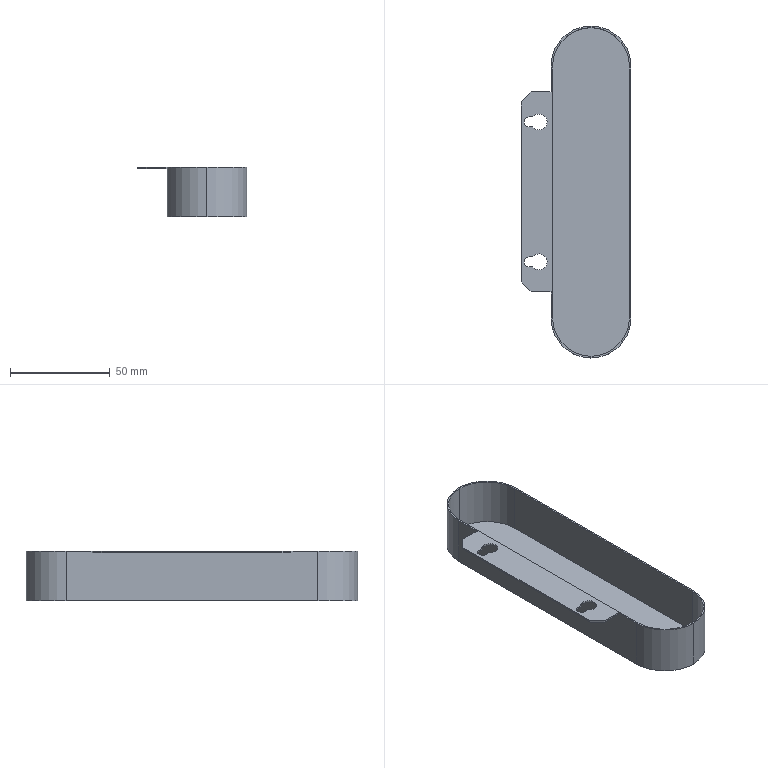Part | NX | features BREP 1 | 1 solid | 31 faces | box 55 x 166 x 25 mm | volume 13374 mm3 | plane 17 | cylinder 14 | commonest cylinder face diameters 5 x4 38.4 x4 40 x4 8 x2
STEP:
#1=CARTESIAN_POINT('',(-31.,-32.5,12.5));
#2=VERTEX_POINT('',#1);
#3=CARTESIAN_POINT('',(-33.5,-35.,12.5));
#4=VERTEX_POINT('',#3);
#5=CARTESIAN_POINT('',(-31.,-35.,12.5));
#6=DIRECTION('',(0.,0.,1.));
#7=DIRECTION('',(-1.,0.,0.));
#8=AXIS2_PLACEMENT_3D('',#5,#6,#7);
#9=CIRCLE('',#8,2.5);
#10=EDGE_CURVE('',#2,#4,#9,.T.);
#11=ORIENTED_EDGE('',*,*,#10,.T.);
#12=CARTESIAN_POINT('',(-33.5,-35.,11.7));
#13=VERTEX_POINT('',#12);
#14=CARTESIAN_POINT('',(-33.5,-35.,12.5));
#15=DIRECTION('',(0.,0.,-1.));
#16=VECTOR('',#15,1000.);
#17=LINE('',#14,#16);
#18=EDGE_CURVE('',#4,#13,#17,.T.);
#19=ORIENTED_EDGE('',*,*,#18,.T.);
#20=CARTESIAN_POINT('',(-31.,-32.5,11.7));
#21=VERTEX_POINT('',#20);
#22=CARTESIAN_POINT('',(-31.,-35.,11.7));
#23=DIRECTION('',(0.,0.,1.));
#24=DIRECTION('',(-1.,0.,0.));
#25=AXIS2_PLACEMENT_3D('',#22,#23,#24);
#26=CIRCLE('',#25,2.5);
#27=EDGE_CURVE('',#21,#13,#26,.T.);
#28=ORIENTED_EDGE('',*,*,#27,.F.);
#29=CARTESIAN_POINT('',(-31.,-32.5,12.5));
#30=DIRECTION('',(0.,0.,-1.));
#31=VECTOR('',#30,1000.);
#32=LINE('',#29,#31);
#33=EDGE_CURVE('',#2,#21,#32,.T.);
#34=ORIENTED_EDGE('',*,*,#33,.F.);
#35=EDGE_LOOP('',(#11,#19,#28,#34));
#36=FACE_BOUND('',#35,.T.);
#37=CARTESIAN_POINT('',(-31.,-35.,12.5));
#38=DIRECTION('',(0.,0.,-1.));
#39=DIRECTION('',(-1.,0.,0.));
#40=AXIS2_PLACEMENT_3D('',#37,#38,#39);
#41=CYLINDRICAL_SURFACE('',#40,2.5);
#42=ADVANCED_FACE('',(#36),#41,.F.);
#43=CARTESIAN_POINT('',(-33.5,35.,12.5));
#44=VERTEX_POINT('',#43);
#45=CARTESIAN_POINT('',(-31.,37.5,12.5));
#46=VERTEX_POINT('',#45);
#47=CARTESIAN_POINT('',(-31.,35.,12.5));
#48=DIRECTION('',(0.,0.,-1.));
#49=DIRECTION('',(-1.,0.,0.));
#50=AXIS2_PLACEMENT_3D('',#47,#48,#49);
#51=CIRCLE('',#50,2.5);
#52=EDGE_CURVE('',#44,#46,#51,.T.);
#53=ORIENTED_EDGE('',*,*,#52,.F.);
#54=CARTESIAN_POINT('',(-33.5,35.,11.7));
#55=VERTEX_POINT('',#54);
#56=CARTESIAN_POINT('',(-33.5,35.,12.5));
#57=DIRECTION('',(0.,0.,-1.));
#58=VECTOR('',#57,1000.);
#59=LINE('',#56,#58);
#60=EDGE_CURVE('',#44,#55,#59,.T.);
#61=ORIENTED_EDGE('',*,*,#60,.T.);
#62=CARTESIAN_POINT('',(-31.,37.5,11.7));
#63=VERTEX_POINT('',#62);
#64=CARTESIAN_POINT('',(-31.,35.,11.7));
#65=DIRECTION('',(0.,0.,-1.));
#66=DIRECTION('',(-1.,0.,0.));
#67=AXIS2_PLACEMENT_3D('',#64,#65,#66);
#68=CIRCLE('',#67,2.5);
#69=EDGE_CURVE('',#55,#63,#68,.T.);
#70=ORIENTED_EDGE('',*,*,#69,.T.);
#71=CARTESIAN_POINT('',(-31.,37.5,12.5));
#72=DIRECTION('',(0.,0.,-1.));
#73=VECTOR('',#72,1000.);
#74=LINE('',#71,#73);
#75=EDGE_CURVE('',#46,#63,#74,.T.);
#76=ORIENTED_EDGE('',*,*,#75,.F.);
#77=EDGE_LOOP('',(#53,#61,#70,#76));
#78=FACE_BOUND('',#77,.T.);
#79=CARTESIAN_POINT('',(-31.,35.,12.5));
#80=DIRECTION('',(0.,0.,-1.));
#81=DIRECTION('',(-1.,0.,0.));
#82=AXIS2_PLACEMENT_3D('',#79,#80,#81);
#83=CYLINDRICAL_SURFACE('',#82,2.5);
#84=ADVANCED_FACE('',(#78),#83,.F.);
#85=CARTESIAN_POINT('',(-35.,-45.,12.5));
#86=VERTEX_POINT('',#85);
#87=CARTESIAN_POINT('',(-35.,45.,12.5));
#88=VERTEX_POINT('',#87);
#89=CARTESIAN_POINT('',(-35.,50.,12.5));
#90=DIRECTION('',(0.,1.,0.));
#91=VECTOR('',#90,1000.);
#92=LINE('',#89,#91);
#93=EDGE_CURVE('',#86,#88,#92,.T.);
#94=ORIENTED_EDGE('',*,*,#93,.F.);
#95=CARTESIAN_POINT('',(-30.,-50.,12.5));
#96=VERTEX_POINT('',#95);
#97=CARTESIAN_POINT('',(-35.,-45.,12.5));
#98=DIRECTION('',(0.7071,-0.7071,0.));
#99=VECTOR('',#98,1000.);
#100=LINE('',#97,#99);
#101=EDGE_CURVE('',#86,#96,#100,.T.);
#102=ORIENTED_EDGE('',*,*,#101,.T.);
#103=CARTESIAN_POINT('',(-20.,-50.,12.5));
#104=VERTEX_POINT('',#103);
#105=CARTESIAN_POINT('',(-35.,-50.,12.5));
#106=DIRECTION('',(1.,0.,0.));
#107=VECTOR('',#106,1000.);
#108=LINE('',#105,#107);
#109=EDGE_CURVE('',#96,#104,#108,.T.);
#110=ORIENTED_EDGE('',*,*,#109,.T.);
#111=CARTESIAN_POINT('',(-20.,-63.,12.5));
#112=VERTEX_POINT('',#111);
#113=CARTESIAN_POINT('',(-20.,83.,12.5));
#114=DIRECTION('',(0.,-1.,0.));
#115=VECTOR('',#114,1000.);
#116=LINE('',#113,#115);
#117=EDGE_CURVE('',#104,#112,#116,.T.);
#118=ORIENTED_EDGE('',*,*,#117,.T.);
#119=CARTESIAN_POINT('',(0.,-83.,12.5));
#120=VERTEX_POINT('',#119);
#121=CARTESIAN_POINT('',(0.,-63.,12.5));
#122=DIRECTION('',(0.,0.,1.));
#123=DIRECTION('',(-1.,0.,0.));
#124=AXIS2_PLACEMENT_3D('',#121,#122,#123);
#125=CIRCLE('',#124,20.);
#126=EDGE_CURVE('',#112,#120,#125,.T.);
#127=ORIENTED_EDGE('',*,*,#126,.T.);
#128=CARTESIAN_POINT('',(20.,-63.,12.5));
#129=VERTEX_POINT('',#128);
#130=CARTESIAN_POINT('',(0.,-63.,12.5));
#131=DIRECTION('',(0.,0.,1.));
#132=DIRECTION('',(-1.,0.,0.));
#133=AXIS2_PLACEMENT_3D('',#130,#131,#132);
#134=CIRCLE('',#133,20.);
#135=EDGE_CURVE('',#120,#129,#134,.T.);
#136=ORIENTED_EDGE('',*,*,#135,.T.);
#137=CARTESIAN_POINT('',(20.,63.,12.5));
#138=VERTEX_POINT('',#137);
#139=CARTESIAN_POINT('',(20.,83.,12.5));
#140=DIRECTION('',(0.,-1.,0.));
#141=VECTOR('',#140,1000.);
#142=LINE('',#139,#141);
#143=EDGE_CURVE('',#138,#129,#142,.T.);
#144=ORIENTED_EDGE('',*,*,#143,.F.);
#145=CARTESIAN_POINT('',(0.,83.,12.5));
#146=VERTEX_POINT('',#145);
#147=CARTESIAN_POINT('',(0.,63.,12.5));
#148=DIRECTION('',(0.,0.,1.));
#149=DIRECTION('',(-1.,0.,0.));
#150=AXIS2_PLACEMENT_3D('',#147,#148,#149);
#151=CIRCLE('',#150,20.);
#152=EDGE_CURVE('',#138,#146,#151,.T.);
#153=ORIENTED_EDGE('',*,*,#152,.T.);
#154=CARTESIAN_POINT('',(-20.,63.,12.5));
#155=VERTEX_POINT('',#154);
#156=CARTESIAN_POINT('',(0.,63.,12.5));
#157=DIRECTION('',(0.,0.,1.));
#158=DIRECTION('',(-1.,0.,0.));
#159=AXIS2_PLACEMENT_3D('',#156,#157,#158);
#160=CIRCLE('',#159,20.);
#161=EDGE_CURVE('',#146,#155,#160,.T.);
#162=ORIENTED_EDGE('',*,*,#161,.T.);
#163=CARTESIAN_POINT('',(-20.,50.,12.5));
#164=VERTEX_POINT('',#163);
#165=CARTESIAN_POINT('',(-20.,83.,12.5));
#166=DIRECTION('',(0.,-1.,0.));
#167=VECTOR('',#166,1000.);
#168=LINE('',#165,#167);
#169=EDGE_CURVE('',#155,#164,#168,.T.);
#170=ORIENTED_EDGE('',*,*,#169,.T.);
#171=CARTESIAN_POINT('',(-30.,50.,12.5));
#172=VERTEX_POINT('',#171);
#173=CARTESIAN_POINT('',(-35.,50.,12.5));
#174=DIRECTION('',(1.,0.,0.));
#175=VECTOR('',#174,1000.);
#176=LINE('',#173,#175);
#177=EDGE_CURVE('',#172,#164,#176,.T.);
#178=ORIENTED_EDGE('',*,*,#177,.F.);
#179=CARTESIAN_POINT('',(-35.,45.,12.5));
#180=DIRECTION('',(-0.7071,-0.7071,0.));
#181=VECTOR('',#180,1000.);
#182=LINE('',#179,#181);
#183=EDGE_CURVE('',#172,#88,#182,.T.);
#184=ORIENTED_EDGE('',*,*,#183,.T.);
#185=EDGE_LOOP('',(#94,#102,#110,#118,#127,#136,#144,#153,#162,#170,#178,#184));
#186=FACE_BOUND('',#185,.T.);
#187=CARTESIAN_POINT('',(-29.122,37.5,12.5));
#188=VERTEX_POINT('',#187);
#189=CARTESIAN_POINT('',(0.,37.5,12.5));
#190=DIRECTION('',(-1.,0.,0.));
#191=VECTOR('',#190,1000.);
#192=LINE('',#189,#191);
#193=EDGE_CURVE('',#188,#46,#192,.T.);
#194=ORIENTED_EDGE('',*,*,#193,.F.);
#195=CARTESIAN_POINT('',(-29.122,32.5,12.5));
#196=VERTEX_POINT('',#195);
#197=CARTESIAN_POINT('',(-26.,35.,12.5));
#198=DIRECTION('',(0.,0.,-1.));
#199=DIRECTION('',(-1.,0.,0.));
#200=AXIS2_PLACEMENT_3D('',#197,#198,#199);
#201=CIRCLE('',#200,4.);
#202=EDGE_CURVE('',#188,#196,#201,.T.);
#203=ORIENTED_EDGE('',*,*,#202,.T.);
#204=CARTESIAN_POINT('',(-31.,32.5,12.5));
#205=VERTEX_POINT('',#204);
#206=CARTESIAN_POINT('',(0.,32.5,12.5));
#207=DIRECTION('',(-1.,0.,0.));
#208=VECTOR('',#207,1000.);
#209=LINE('',#206,#208);
#210=EDGE_CURVE('',#196,#205,#209,.T.);
#211=ORIENTED_EDGE('',*,*,#210,.T.);
#212=CARTESIAN_POINT('',(-31.,35.,12.5));
#213=DIRECTION('',(0.,0.,-1.));
#214=DIRECTION('',(-1.,0.,0.));
#215=AXIS2_PLACEMENT_3D('',#212,#213,#214);
#216=CIRCLE('',#215,2.5);
#217=EDGE_CURVE('',#205,#44,#216,.T.);
#218=ORIENTED_EDGE('',*,*,#217,.T.);
#219=ORIENTED_EDGE('',*,*,#52,.T.);
#220=EDGE_LOOP('',(#194,#203,#211,#218,#219));
#221=FACE_BOUND('',#220,.T.);
#222=CARTESIAN_POINT('',(-19.2,-63.,12.5));
#223=VERTEX_POINT('',#222);
#224=CARTESIAN_POINT('',(0.,-82.2,12.5));
#225=VERTEX_POINT('',#224);
#226=CARTESIAN_POINT('',(0.,-63.,12.5));
#227=DIRECTION('',(0.,0.,1.));
#228=DIRECTION('',(-1.,0.,0.));
#229=AXIS2_PLACEMENT_3D('',#226,#227,#228);
#230=CIRCLE('',#229,19.2);
#231=EDGE_CURVE('',#223,#225,#230,.T.);
#232=ORIENTED_EDGE('',*,*,#231,.F.);
#233=CARTESIAN_POINT('',(-19.2,63.,12.5));
#234=VERTEX_POINT('',#233);
#235=CARTESIAN_POINT('',(-19.2,83.,12.5));
#236=DIRECTION('',(0.,-1.,0.));
#237=VECTOR('',#236,1000.);
#238=LINE('',#235,#237);
#239=EDGE_CURVE('',#234,#223,#238,.T.);
#240=ORIENTED_EDGE('',*,*,#239,.F.);
#241=CARTESIAN_POINT('',(0.,82.2,12.5));
#242=VERTEX_POINT('',#241);
#243=CARTESIAN_POINT('',(0.,63.,12.5));
#244=DIRECTION('',(0.,0.,1.));
#245=DIRECTION('',(-1.,0.,0.));
#246=AXIS2_PLACEMENT_3D('',#243,#244,#245);
#247=CIRCLE('',#246,19.2);
#248=EDGE_CURVE('',#242,#234,#247,.T.);
#249=ORIENTED_EDGE('',*,*,#248,.F.);
#250=CARTESIAN_POINT('',(19.2,63.,12.5));
#251=VERTEX_POINT('',#250);
#252=CARTESIAN_POINT('',(0.,63.,12.5));
#253=DIRECTION('',(0.,0.,1.));
#254=DIRECTION('',(-1.,0.,0.));
#255=AXIS2_PLACEMENT_3D('',#252,#253,#254);
#256=CIRCLE('',#255,19.2);
#257=EDGE_CURVE('',#251,#242,#256,.T.);
#258=ORIENTED_EDGE('',*,*,#257,.F.);
#259=CARTESIAN_POINT('',(19.2,-63.,12.5));
#260=VERTEX_POINT('',#259);
#261=CARTESIAN_POINT('',(19.2,83.,12.5));
#262=DIRECTION('',(0.,-1.,0.));
#263=VECTOR('',#262,1000.);
#264=LINE('',#261,#263);
#265=EDGE_CURVE('',#251,#260,#264,.T.);
#266=ORIENTED_EDGE('',*,*,#265,.T.);
#267=CARTESIAN_POINT('',(0.,-63.,12.5));
#268=DIRECTION('',(0.,0.,1.));
#269=DIRECTION('',(-1.,0.,0.));
#270=AXIS2_PLACEMENT_3D('',#267,#268,#269);
#271=CIRCLE('',#270,19.2);
#272=EDGE_CURVE('',#225,#260,#271,.T.);
#273=ORIENTED_EDGE('',*,*,#272,.F.);
#274=EDGE_LOOP('',(#232,#240,#249,#258,#266,#273));
#275=FACE_BOUND('',#274,.T.);
#276=CARTESIAN_POINT('',(-29.122,-32.5,12.5));
#277=VERTEX_POINT('',#276);
#278=CARTESIAN_POINT('',(0.,-32.5,12.5));
#279=DIRECTION('',(-1.,0.,0.));
#280=VECTOR('',#279,1000.);
#281=LINE('',#278,#280);
#282=EDGE_CURVE('',#277,#2,#281,.T.);
#283=ORIENTED_EDGE('',*,*,#282,.F.);
#284=CARTESIAN_POINT('',(-29.122,-37.5,12.5));
#285=VERTEX_POINT('',#284);
#286=CARTESIAN_POINT('',(-26.,-35.,12.5));
#287=DIRECTION('',(0.,0.,1.));
#288=DIRECTION('',(-1.,0.,0.));
#289=AXIS2_PLACEMENT_3D('',#286,#287,#288);
#290=CIRCLE('',#289,4.);
#291=EDGE_CURVE('',#285,#277,#290,.T.);
#292=ORIENTED_EDGE('',*,*,#291,.F.);
#293=CARTESIAN_POINT('',(-31.,-37.5,12.5));
#294=VERTEX_POINT('',#293);
#295=CARTESIAN_POINT('',(0.,-37.5,12.5));
#296=DIRECTION('',(-1.,0.,0.));
#297=VECTOR('',#296,1000.);
#298=LINE('',#295,#297);
#299=EDGE_CURVE('',#285,#294,#298,.T.);
#300=ORIENTED_EDGE('',*,*,#299,.T.);
#301=CARTESIAN_POINT('',(-31.,-35.,12.5));
#302=DIRECTION('',(0.,0.,1.));
#303=DIRECTION('',(-1.,0.,0.));
#304=AXIS2_PLACEMENT_3D('',#301,#302,#303);
#305=CIRCLE('',#304,2.5);
#306=EDGE_CURVE('',#4,#294,#305,.T.);
#307=ORIENTED_EDGE('',*,*,#306,.F.);
#308=ORIENTED_EDGE('',*,*,#10,.F.);
#309=EDGE_LOOP('',(#283,#292,#300,#307,#308));
#310=FACE_BOUND('',#309,.T.);
#311=CARTESIAN_POINT('',(-20.,83.,12.5));
#312=DIRECTION('',(0.,0.,-1.));
#313=DIRECTION('',(0.,-1.,0.));
#314=AXIS2_PLACEMENT_3D('',#311,#312,#313);
#315=PLANE('',#314);
#316=ADVANCED_FACE('',(#186,#221,#275,#310),#315,.F.);
#317=CARTESIAN_POINT('',(-30.,-50.,11.7));
#318=VERTEX_POINT('',#317);
#319=CARTESIAN_POINT('',(-20.,-50.,11.7));
#320=VERTEX_POINT('',#319);
#321=CARTESIAN_POINT('',(-35.,-50.,11.7));
#322=DIRECTION('',(1.,0.,0.));
#323=VECTOR('',#322,1000.);
#324=LINE('',#321,#323);
#325=EDGE_CURVE('',#318,#320,#324,.T.);
#326=ORIENTED_EDGE('',*,*,#325,.F.);
#327=CARTESIAN_POINT('',(-35.,-45.,11.7));
#328=VERTEX_POINT('',#327);
#329=CARTESIAN_POINT('',(-35.,-45.,11.7));
#330=DIRECTION('',(-0.7071,0.7071,0.));
#331=VECTOR('',#330,1000.);
#332=LINE('',#329,#331);
#333=EDGE_CURVE('',#318,#328,#332,.T.);
#334=ORIENTED_EDGE('',*,*,#333,.T.);
#335=CARTESIAN_POINT('',(-35.,45.,11.7));
#336=VERTEX_POINT('',#335);
#337=CARTESIAN_POINT('',(-35.,50.,11.7));
#338=DIRECTION('',(0.,-1.,0.));
#339=VECTOR('',#338,1000.);
#340=LINE('',#337,#339);
#341=EDGE_CURVE('',#336,#328,#340,.T.);
#342=ORIENTED_EDGE('',*,*,#341,.F.);
#343=CARTESIAN_POINT('',(-30.,50.,11.7));
#344=VERTEX_POINT('',#343);
#345=CARTESIAN_POINT('',(-35.,45.,11.7));
#346=DIRECTION('',(0.7071,0.7071,0.));
#347=VECTOR('',#346,1000.);
#348=LINE('',#345,#347);
#349=EDGE_CURVE('',#336,#344,#348,.T.);
#350=ORIENTED_EDGE('',*,*,#349,.T.);
#351=CARTESIAN_POINT('',(-20.,50.,11.7));
#352=VERTEX_POINT('',#351);
#353=CARTESIAN_POINT('',(-35.,50.,11.7));
#354=DIRECTION('',(1.,0.,0.));
#355=VECTOR('',#354,1000.);
#356=LINE('',#353,#355);
#357=EDGE_CURVE('',#344,#352,#356,.T.);
#358=ORIENTED_EDGE('',*,*,#357,.T.);
#359=CARTESIAN_POINT('',(-20.,50.,11.7));
#360=DIRECTION('',(0.,-1.,0.));
#361=VECTOR('',#360,1000.);
#362=LINE('',#359,#361);
#363=EDGE_CURVE('',#352,#320,#362,.T.);
#364=ORIENTED_EDGE('',*,*,#363,.T.);
#365=EDGE_LOOP('',(#326,#334,#342,#350,#358,#364));
#366=FACE_BOUND('',#365,.T.);
#367=CARTESIAN_POINT('',(-29.122,37.5,11.7));
#368=VERTEX_POINT('',#367);
#369=CARTESIAN_POINT('',(0.,37.5,11.7));
#370=DIRECTION('',(-1.,0.,0.));
#371=VECTOR('',#370,1000.);
#372=LINE('',#369,#371);
#373=EDGE_CURVE('',#368,#63,#372,.T.);
#374=ORIENTED_EDGE('',*,*,#373,.T.);
#375=ORIENTED_EDGE('',*,*,#69,.F.);
#376=CARTESIAN_POINT('',(-31.,32.5,11.7));
#377=VERTEX_POINT('',#376);
#378=CARTESIAN_POINT('',(-31.,35.,11.7));
#379=DIRECTION('',(0.,0.,-1.));
#380=DIRECTION('',(-1.,0.,0.));
#381=AXIS2_PLACEMENT_3D('',#378,#379,#380);
#382=CIRCLE('',#381,2.5);
#383=EDGE_CURVE('',#377,#55,#382,.T.);
#384=ORIENTED_EDGE('',*,*,#383,.F.);
#385=CARTESIAN_POINT('',(-29.122,32.5,11.7));
#386=VERTEX_POINT('',#385);
#387=CARTESIAN_POINT('',(0.,32.5,11.7));
#388=DIRECTION('',(-1.,0.,0.));
#389=VECTOR('',#388,1000.);
#390=LINE('',#387,#389);
#391=EDGE_CURVE('',#386,#377,#390,.T.);
#392=ORIENTED_EDGE('',*,*,#391,.F.);
#393=CARTESIAN_POINT('',(-26.,35.,11.7));
#394=DIRECTION('',(0.,0.,-1.));
#395=DIRECTION('',(-1.,0.,0.));
#396=AXIS2_PLACEMENT_3D('',#393,#394,#395);
#397=CIRCLE('',#396,4.);
#398=EDGE_CURVE('',#368,#386,#397,.T.);
#399=ORIENTED_EDGE('',*,*,#398,.F.);
#400=EDGE_LOOP('',(#374,#375,#384,#392,#399));
#401=FACE_BOUND('',#400,.T.);
#402=CARTESIAN_POINT('',(-29.122,-32.5,11.7));
#403=VERTEX_POINT('',#402);
#404=CARTESIAN_POINT('',(0.,-32.5,11.7));
#405=DIRECTION('',(-1.,0.,0.));
#406=VECTOR('',#405,1000.);
#407=LINE('',#404,#406);
#408=EDGE_CURVE('',#403,#21,#407,.T.);
#409=ORIENTED_EDGE('',*,*,#408,.T.);
#410=ORIENTED_EDGE('',*,*,#27,.T.);
#411=CARTESIAN_POINT('',(-31.,-37.5,11.7));
#412=VERTEX_POINT('',#411);
#413=CARTESIAN_POINT('',(-31.,-35.,11.7));
#414=DIRECTION('',(0.,0.,1.));
#415=DIRECTION('',(-1.,0.,0.));
#416=AXIS2_PLACEMENT_3D('',#413,#414,#415);
#417=CIRCLE('',#416,2.5);
#418=EDGE_CURVE('',#13,#412,#417,.T.);
#419=ORIENTED_EDGE('',*,*,#418,.T.);
#420=CARTESIAN_POINT('',(-29.122,-37.5,11.7));
#421=VERTEX_POINT('',#420);
#422=CARTESIAN_POINT('',(0.,-37.5,11.7));
#423=DIRECTION('',(-1.,0.,0.));
#424=VECTOR('',#423,1000.);
#425=LINE('',#422,#424);
#426=EDGE_CURVE('',#421,#412,#425,.T.);
#427=ORIENTED_EDGE('',*,*,#426,.F.);
#428=CARTESIAN_POINT('',(-26.,-35.,11.7));
#429=DIRECTION('',(0.,0.,1.));
#430=DIRECTION('',(-1.,0.,0.));
#431=AXIS2_PLACEMENT_3D('',#428,#429,#430);
#432=CIRCLE('',#431,4.);
#433=EDGE_CURVE('',#421,#403,#432,.T.);
#434=ORIENTED_EDGE('',*,*,#433,.T.);
#435=EDGE_LOOP('',(#409,#410,#419,#427,#434));
#436=FACE_BOUND('',#435,.T.);
#437=CARTESIAN_POINT('',(-35.,50.,11.7));
#438=DIRECTION('',(0.,0.,1.));
#439=DIRECTION('',(1.,0.,0.));
#440=AXIS2_PLACEMENT_3D('',#437,#438,#439);
#441=PLANE('',#440);
#442=ADVANCED_FACE('',(#366,#401,#436),#441,.F.);
#443=CARTESIAN_POINT('',(-20.,50.,12.5));
#444=DIRECTION('',(0.,0.,-1.));
#445=VECTOR('',#444,1000.);
#446=LINE('',#443,#445);
#447=EDGE_CURVE('',#164,#352,#446,.T.);
#448=ORIENTED_EDGE('',*,*,#447,.F.);
#449=ORIENTED_EDGE('',*,*,#169,.F.);
#450=CARTESIAN_POINT('',(-20.,63.,-12.5));
#451=VERTEX_POINT('',#450);
#452=CARTESIAN_POINT('',(-20.,63.,-12.5));
#453=DIRECTION('',(0.,0.,-1.));
#454=VECTOR('',#453,1000.);
#455=LINE('',#452,#454);
#456=EDGE_CURVE('',#155,#451,#455,.T.);
#457=ORIENTED_EDGE('',*,*,#456,.T.);
#458=CARTESIAN_POINT('',(-20.,-63.,-12.5));
#459=VERTEX_POINT('',#458);
#460=CARTESIAN_POINT('',(-20.,83.,-12.5));
#461=DIRECTION('',(0.,-1.,0.));
#462=VECTOR('',#461,1000.);
#463=LINE('',#460,#462);
#464=EDGE_CURVE('',#451,#459,#463,.T.);
#465=ORIENTED_EDGE('',*,*,#464,.T.);
#466=CARTESIAN_POINT('',(-20.,-63.,-12.5));
#467=DIRECTION('',(0.,0.,1.));
#468=VECTOR('',#467,1000.);
#469=LINE('',#466,#468);
#470=EDGE_CURVE('',#459,#112,#469,.T.);
#471=ORIENTED_EDGE('',*,*,#470,.T.);
#472=ORIENTED_EDGE('',*,*,#117,.F.);
#473=CARTESIAN_POINT('',(-20.,-50.,12.5));
#474=DIRECTION('',(0.,0.,1.));
#475=VECTOR('',#474,1000.);
#476=LINE('',#473,#475);
#477=EDGE_CURVE('',#320,#104,#476,.T.);
#478=ORIENTED_EDGE('',*,*,#477,.F.);
#479=ORIENTED_EDGE('',*,*,#363,.F.);
#480=EDGE_LOOP('',(#448,#449,#457,#465,#471,#472,#478,#479));
#481=FACE_BOUND('',#480,.T.);
#482=CARTESIAN_POINT('',(-20.,83.,-12.5));
#483=DIRECTION('',(1.,0.,0.));
#484=DIRECTION('',(0.,1.,0.));
#485=AXIS2_PLACEMENT_3D('',#482,#483,#484);
#486=PLANE('',#485);
#487=ADVANCED_FACE('',(#481),#486,.F.);
#488=ORIENTED_EDGE('',*,*,#143,.T.);
#489=CARTESIAN_POINT('',(20.,-63.,-12.5));
#490=VERTEX_POINT('',#489);
#491=CARTESIAN_POINT('',(20.,-63.,-12.5));
#492=DIRECTION('',(0.,0.,-1.));
#493=VECTOR('',#492,1000.);
#494=LINE('',#491,#493);
#495=EDGE_CURVE('',#129,#490,#494,.T.);
#496=ORIENTED_EDGE('',*,*,#495,.T.);
#497=CARTESIAN_POINT('',(20.,63.,-12.5));
#498=VERTEX_POINT('',#497);
#499=CARTESIAN_POINT('',(20.,83.,-12.5));
#500=DIRECTION('',(0.,-1.,0.));
#501=VECTOR('',#500,1000.);
#502=LINE('',#499,#501);
#503=EDGE_CURVE('',#498,#490,#502,.T.);
#504=ORIENTED_EDGE('',*,*,#503,.F.);
#505=CARTESIAN_POINT('',(20.,63.,12.5));
#506=DIRECTION('',(0.,0.,1.));
#507=VECTOR('',#506,1000.);
#508=LINE('',#505,#507);
#509=EDGE_CURVE('',#498,#138,#508,.T.);
#510=ORIENTED_EDGE('',*,*,#509,.T.);
#511=EDGE_LOOP('',(#488,#496,#504,#510));
#512=FACE_BOUND('',#511,.T.);
#513=CARTESIAN_POINT('',(20.,83.,-12.5));
#514=DIRECTION('',(-1.,0.,0.));
#515=DIRECTION('',(0.,0.,1.));
#516=AXIS2_PLACEMENT_3D('',#513,#514,#515);
#517=PLANE('',#516);
#518=ADVANCED_FACE('',(#512),#517,.F.);
#519=ORIENTED_EDGE('',*,*,#503,.T.);
#520=CARTESIAN_POINT('',(0.,-83.,-12.5));
#521=VERTEX_POINT('',#520);
#522=CARTESIAN_POINT('',(0.,-63.,-12.5));
#523=DIRECTION('',(0.,0.,-1.));
#524=DIRECTION('',(1.,0.,0.));
#525=AXIS2_PLACEMENT_3D('',#522,#523,#524);
#526=CIRCLE('',#525,20.);
#527=EDGE_CURVE('',#490,#521,#526,.T.);
#528=ORIENTED_EDGE('',*,*,#527,.T.);
#529=CARTESIAN_POINT('',(0.,-63.,-12.5));
#530=DIRECTION('',(0.,0.,-1.));
#531=DIRECTION('',(1.,0.,0.));
#532=AXIS2_PLACEMENT_3D('',#529,#530,#531);
#533=CIRCLE('',#532,20.);
#534=EDGE_CURVE('',#521,#459,#533,.T.);
#535=ORIENTED_EDGE('',*,*,#534,.T.);
#536=ORIENTED_EDGE('',*,*,#464,.F.);
#537=CARTESIAN_POINT('',(0.,83.,-12.5));
#538=VERTEX_POINT('',#537);
#539=CARTESIAN_POINT('',(0.,63.,-12.5));
#540=DIRECTION('',(0.,0.,-1.));
#541=DIRECTION('',(1.,0.,0.));
#542=AXIS2_PLACEMENT_3D('',#539,#540,#541);
#543=CIRCLE('',#542,20.);
#544=EDGE_CURVE('',#451,#538,#543,.T.);
#545=ORIENTED_EDGE('',*,*,#544,.T.);
#546=CARTESIAN_POINT('',(0.,63.,-12.5));
#547=DIRECTION('',(0.,0.,-1.));
#548=DIRECTION('',(1.,0.,0.));
#549=AXIS2_PLACEMENT_3D('',#546,#547,#548);
#550=CIRCLE('',#549,20.);
#551=EDGE_CURVE('',#538,#498,#550,.T.);
#552=ORIENTED_EDGE('',*,*,#551,.T.);
#553=EDGE_LOOP('',(#519,#528,#535,#536,#545,#552));
#554=FACE_BOUND('',#553,.T.);
#555=CARTESIAN_POINT('',(-20.,83.,-12.5));
#556=DIRECTION('',(0.,0.,1.));
#557=DIRECTION('',(1.,0.,0.));
#558=AXIS2_PLACEMENT_3D('',#555,#556,#557);
#559=PLANE('',#558);
#560=ADVANCED_FACE('',(#554),#559,.F.);
#561=CARTESIAN_POINT('',(0.,-83.,12.5));
#562=DIRECTION('',(0.,0.,-1.));
#563=VECTOR('',#562,1000.);
#564=LINE('',#561,#563);
#565=EDGE_CURVE('',#120,#521,#564,.T.);
#566=ORIENTED_EDGE('',*,*,#565,.F.);
#567=ORIENTED_EDGE('',*,*,#126,.F.);
#568=ORIENTED_EDGE('',*,*,#470,.F.);
#569=ORIENTED_EDGE('',*,*,#534,.F.);
#570=EDGE_LOOP('',(#566,#567,#568,#569));
#571=FACE_BOUND('',#570,.T.);
#572=CARTESIAN_POINT('',(0.,-63.,-12.5));
#573=DIRECTION('',(0.,0.,1.));
#574=DIRECTION('',(1.,0.,0.));
#575=AXIS2_PLACEMENT_3D('',#572,#573,#574);
#576=CYLINDRICAL_SURFACE('',#575,20.);
#577=ADVANCED_FACE('',(#571),#576,.T.);
#578=ORIENTED_EDGE('',*,*,#135,.F.);
#579=ORIENTED_EDGE('',*,*,#565,.T.);
#580=ORIENTED_EDGE('',*,*,#527,.F.);
#581=ORIENTED_EDGE('',*,*,#495,.F.);
#582=EDGE_LOOP('',(#578,#579,#580,#581));
#583=FACE_BOUND('',#582,.T.);
#584=CARTESIAN_POINT('',(0.,-63.,-12.5));
#585=DIRECTION('',(0.,0.,-1.));
#586=DIRECTION('',(-1.,0.,0.));
#587=AXIS2_PLACEMENT_3D('',#584,#585,#586);
#588=CYLINDRICAL_SURFACE('',#587,20.);
#589=ADVANCED_FACE('',(#583),#588,.T.);
#590=ORIENTED_EDGE('',*,*,#456,.F.);
#591=ORIENTED_EDGE('',*,*,#161,.F.);
#592=CARTESIAN_POINT('',(0.,83.,12.5));
#593=DIRECTION('',(0.,0.,1.));
#594=VECTOR('',#593,1000.);
#595=LINE('',#592,#594);
#596=EDGE_CURVE('',#538,#146,#595,.T.);
#597=ORIENTED_EDGE('',*,*,#596,.F.);
#598=ORIENTED_EDGE('',*,*,#544,.F.);
#599=EDGE_LOOP('',(#590,#591,#597,#598));
#600=FACE_BOUND('',#599,.T.);
#601=CARTESIAN_POINT('',(0.,63.,12.5));
#602=DIRECTION('',(0.,0.,-1.));
#603=DIRECTION('',(-1.,0.,0.));
#604=AXIS2_PLACEMENT_3D('',#601,#602,#603);
#605=CYLINDRICAL_SURFACE('',#604,20.);
#606=ADVANCED_FACE('',(#600),#605,.T.);
#607=ORIENTED_EDGE('',*,*,#152,.F.);
#608=ORIENTED_EDGE('',*,*,#509,.F.);
#609=ORIENTED_EDGE('',*,*,#551,.F.);
#610=ORIENTED_EDGE('',*,*,#596,.T.);
#611=EDGE_LOOP('',(#607,#608,#609,#610));
#612=FACE_BOUND('',#611,.T.);
#613=CARTESIAN_POINT('',(0.,63.,12.5));
#614=DIRECTION('',(0.,0.,1.));
#615=DIRECTION('',(1.,0.,0.));
#616=AXIS2_PLACEMENT_3D('',#613,#614,#615);
#617=CYLINDRICAL_SURFACE('',#616,20.);
#618=ADVANCED_FACE('',(#612),#617,.T.);
#619=CARTESIAN_POINT('',(-19.2,63.,-11.7));
#620=VERTEX_POINT('',#619);
#621=CARTESIAN_POINT('',(-19.2,-63.,-11.7));
#622=VERTEX_POINT('',#621);
#623=CARTESIAN_POINT('',(-19.2,83.,-11.7));
#624=DIRECTION('',(0.,-1.,0.));
#625=VECTOR('',#624,1000.);
#626=LINE('',#623,#625);
#627=EDGE_CURVE('',#620,#622,#626,.T.);
#628=ORIENTED_EDGE('',*,*,#627,.F.);
#629=CARTESIAN_POINT('',(-19.2,63.,-12.5));
#630=DIRECTION('',(0.,0.,-1.));
#631=VECTOR('',#630,1000.);
#632=LINE('',#629,#631);
#633=EDGE_CURVE('',#234,#620,#632,.T.);
#634=ORIENTED_EDGE('',*,*,#633,.F.);
#635=ORIENTED_EDGE('',*,*,#239,.T.);
#636=CARTESIAN_POINT('',(-19.2,-63.,-12.5));
#637=DIRECTION('',(0.,0.,1.));
#638=VECTOR('',#637,1000.);
#639=LINE('',#636,#638);
#640=EDGE_CURVE('',#622,#223,#639,.T.);
#641=ORIENTED_EDGE('',*,*,#640,.F.);
#642=EDGE_LOOP('',(#628,#634,#635,#641));
#643=FACE_BOUND('',#642,.T.);
#644=CARTESIAN_POINT('',(-19.2,83.,-12.5));
#645=DIRECTION('',(1.,0.,0.));
#646=DIRECTION('',(0.,1.,0.));
#647=AXIS2_PLACEMENT_3D('',#644,#645,#646);
#648=PLANE('',#647);
#649=ADVANCED_FACE('',(#643),#648,.T.);
#650=ORIENTED_EDGE('',*,*,#265,.F.);
#651=CARTESIAN_POINT('',(19.2,63.,-11.7));
#652=VERTEX_POINT('',#651);
#653=CARTESIAN_POINT('',(19.2,63.,-12.5));
#654=DIRECTION('',(0.,0.,1.));
#655=VECTOR('',#654,1000.);
#656=LINE('',#653,#655);
#657=EDGE_CURVE('',#652,#251,#656,.T.);
#658=ORIENTED_EDGE('',*,*,#657,.F.);
#659=CARTESIAN_POINT('',(19.2,-63.,-11.7));
#660=VERTEX_POINT('',#659);
#661=CARTESIAN_POINT('',(19.2,83.,-11.7));
#662=DIRECTION('',(0.,-1.,0.));
#663=VECTOR('',#662,1000.);
#664=LINE('',#661,#663);
#665=EDGE_CURVE('',#652,#660,#664,.T.);
#666=ORIENTED_EDGE('',*,*,#665,.T.);
#667=CARTESIAN_POINT('',(19.2,-63.,-12.5));
#668=DIRECTION('',(0.,0.,-1.));
#669=VECTOR('',#668,1000.);
#670=LINE('',#667,#669);
#671=EDGE_CURVE('',#260,#660,#670,.T.);
#672=ORIENTED_EDGE('',*,*,#671,.F.);
#673=EDGE_LOOP('',(#650,#658,#666,#672));
#674=FACE_BOUND('',#673,.T.);
#675=CARTESIAN_POINT('',(19.2,83.,-12.5));
#676=DIRECTION('',(-1.,0.,0.));
#677=DIRECTION('',(0.,0.,1.));
#678=AXIS2_PLACEMENT_3D('',#675,#676,#677);
#679=PLANE('',#678);
#680=ADVANCED_FACE('',(#674),#679,.T.);
#681=ORIENTED_EDGE('',*,*,#665,.F.);
#682=CARTESIAN_POINT('',(0.,82.2,-11.7));
#683=VERTEX_POINT('',#682);
#684=CARTESIAN_POINT('',(0.,63.,-11.7));
#685=DIRECTION('',(0.,0.,-1.));
#686=DIRECTION('',(1.,0.,0.));
#687=AXIS2_PLACEMENT_3D('',#684,#685,#686);
#688=CIRCLE('',#687,19.2);
#689=EDGE_CURVE('',#683,#652,#688,.T.);
#690=ORIENTED_EDGE('',*,*,#689,.F.);
#691=CARTESIAN_POINT('',(0.,63.,-11.7));
#692=DIRECTION('',(0.,0.,-1.));
#693=DIRECTION('',(1.,0.,0.));
#694=AXIS2_PLACEMENT_3D('',#691,#692,#693);
#695=CIRCLE('',#694,19.2);
#696=EDGE_CURVE('',#620,#683,#695,.T.);
#697=ORIENTED_EDGE('',*,*,#696,.F.);
#698=ORIENTED_EDGE('',*,*,#627,.T.);
#699=CARTESIAN_POINT('',(0.,-82.2,-11.7));
#700=VERTEX_POINT('',#699);
#701=CARTESIAN_POINT('',(0.,-63.,-11.7));
#702=DIRECTION('',(0.,0.,-1.));
#703=DIRECTION('',(1.,0.,0.));
#704=AXIS2_PLACEMENT_3D('',#701,#702,#703);
#705=CIRCLE('',#704,19.2);
#706=EDGE_CURVE('',#700,#622,#705,.T.);
#707=ORIENTED_EDGE('',*,*,#706,.F.);
#708=CARTESIAN_POINT('',(0.,-63.,-11.7));
#709=DIRECTION('',(0.,0.,-1.));
#710=DIRECTION('',(1.,0.,0.));
#711=AXIS2_PLACEMENT_3D('',#708,#709,#710);
#712=CIRCLE('',#711,19.2);
#713=EDGE_CURVE('',#660,#700,#712,.T.);
#714=ORIENTED_EDGE('',*,*,#713,.F.);
#715=EDGE_LOOP('',(#681,#690,#697,#698,#707,#714));
#716=FACE_BOUND('',#715,.T.);
#717=CARTESIAN_POINT('',(-20.,83.,-11.7));
#718=DIRECTION('',(0.,0.,1.));
#719=DIRECTION('',(1.,0.,0.));
#720=AXIS2_PLACEMENT_3D('',#717,#718,#719);
#721=PLANE('',#720);
#722=ADVANCED_FACE('',(#716),#721,.T.);
#723=CARTESIAN_POINT('',(0.,-82.2,-12.5));
#724=DIRECTION('',(0.,0.,-1.));
#725=VECTOR('',#724,1000.);
#726=LINE('',#723,#725);
#727=EDGE_CURVE('',#225,#700,#726,.T.);
#728=ORIENTED_EDGE('',*,*,#727,.T.);
#729=ORIENTED_EDGE('',*,*,#706,.T.);
#730=ORIENTED_EDGE('',*,*,#640,.T.);
#731=ORIENTED_EDGE('',*,*,#231,.T.);
#732=EDGE_LOOP('',(#728,#729,#730,#731));
#733=FACE_BOUND('',#732,.T.);
#734=CARTESIAN_POINT('',(0.,-63.,-12.5));
#735=DIRECTION('',(0.,0.,1.));
#736=DIRECTION('',(1.,0.,0.));
#737=AXIS2_PLACEMENT_3D('',#734,#735,#736);
#738=CYLINDRICAL_SURFACE('',#737,19.2);
#739=ADVANCED_FACE('',(#733),#738,.F.);
#740=ORIENTED_EDGE('',*,*,#272,.T.);
#741=ORIENTED_EDGE('',*,*,#671,.T.);
#742=ORIENTED_EDGE('',*,*,#713,.T.);
#743=ORIENTED_EDGE('',*,*,#727,.F.);
#744=EDGE_LOOP('',(#740,#741,#742,#743));
#745=FACE_BOUND('',#744,.T.);
#746=CARTESIAN_POINT('',(0.,-63.,-12.5));
#747=DIRECTION('',(0.,0.,-1.));
#748=DIRECTION('',(-1.,0.,0.));
#749=AXIS2_PLACEMENT_3D('',#746,#747,#748);
#750=CYLINDRICAL_SURFACE('',#749,19.2);
#751=ADVANCED_FACE('',(#745),#750,.F.);
#752=ORIENTED_EDGE('',*,*,#633,.T.);
#753=ORIENTED_EDGE('',*,*,#696,.T.);
#754=CARTESIAN_POINT('',(0.,82.2,12.5));
#755=DIRECTION('',(0.,0.,1.));
#756=VECTOR('',#755,1000.);
#757=LINE('',#754,#756);
#758=EDGE_CURVE('',#683,#242,#757,.T.);
#759=ORIENTED_EDGE('',*,*,#758,.T.);
#760=ORIENTED_EDGE('',*,*,#248,.T.);
#761=EDGE_LOOP('',(#752,#753,#759,#760));
#762=FACE_BOUND('',#761,.T.);
#763=CARTESIAN_POINT('',(0.,63.,12.5));
#764=DIRECTION('',(0.,0.,-1.));
#765=DIRECTION('',(-1.,0.,0.));
#766=AXIS2_PLACEMENT_3D('',#763,#764,#765);
#767=CYLINDRICAL_SURFACE('',#766,19.2);
#768=ADVANCED_FACE('',(#762),#767,.F.);
#769=ORIENTED_EDGE('',*,*,#257,.T.);
#770=ORIENTED_EDGE('',*,*,#758,.F.);
#771=ORIENTED_EDGE('',*,*,#689,.T.);
#772=ORIENTED_EDGE('',*,*,#657,.T.);
#773=EDGE_LOOP('',(#769,#770,#771,#772));
#774=FACE_BOUND('',#773,.T.);
#775=CARTESIAN_POINT('',(0.,63.,12.5));
#776=DIRECTION('',(0.,0.,1.));
#777=DIRECTION('',(1.,0.,0.));
#778=AXIS2_PLACEMENT_3D('',#775,#776,#777);
#779=CYLINDRICAL_SURFACE('',#778,19.2);
#780=ADVANCED_FACE('',(#774),#779,.F.);
#781=ORIENTED_EDGE('',*,*,#357,.F.);
#782=CARTESIAN_POINT('',(-30.,50.,12.5));
#783=DIRECTION('',(0.,0.,1.));
#784=VECTOR('',#783,1000.);
#785=LINE('',#782,#784);
#786=EDGE_CURVE('',#344,#172,#785,.T.);
#787=ORIENTED_EDGE('',*,*,#786,.T.);
#788=ORIENTED_EDGE('',*,*,#177,.T.);
#789=ORIENTED_EDGE('',*,*,#447,.T.);
#790=EDGE_LOOP('',(#781,#787,#788,#789));
#791=FACE_BOUND('',#790,.T.);
#792=CARTESIAN_POINT('',(-35.,50.,12.5));
#793=DIRECTION('',(0.,-1.,0.));
#794=DIRECTION('',(0.,0.,-1.));
#795=AXIS2_PLACEMENT_3D('',#792,#793,#794);
#796=PLANE('',#795);
#797=ADVANCED_FACE('',(#791),#796,.F.);
#798=ORIENTED_EDGE('',*,*,#109,.F.);
#799=CARTESIAN_POINT('',(-30.,-50.,12.5));
#800=DIRECTION('',(0.,0.,-1.));
#801=VECTOR('',#800,1000.);
#802=LINE('',#799,#801);
#803=EDGE_CURVE('',#96,#318,#802,.T.);
#804=ORIENTED_EDGE('',*,*,#803,.T.);
#805=ORIENTED_EDGE('',*,*,#325,.T.);
#806=ORIENTED_EDGE('',*,*,#477,.T.);
#807=EDGE_LOOP('',(#798,#804,#805,#806));
#808=FACE_BOUND('',#807,.T.);
#809=CARTESIAN_POINT('',(-35.,-50.,12.5));
#810=DIRECTION('',(0.,1.,0.));
#811=DIRECTION('',(1.,0.,0.));
#812=AXIS2_PLACEMENT_3D('',#809,#810,#811);
#813=PLANE('',#812);
#814=ADVANCED_FACE('',(#808),#813,.F.);
#815=ORIENTED_EDGE('',*,*,#341,.T.);
#816=CARTESIAN_POINT('',(-35.,-45.,0.));
#817=DIRECTION('',(0.,0.,1.));
#818=VECTOR('',#817,1000.);
#819=LINE('',#816,#818);
#820=EDGE_CURVE('',#328,#86,#819,.T.);
#821=ORIENTED_EDGE('',*,*,#820,.T.);
#822=ORIENTED_EDGE('',*,*,#93,.T.);
#823=CARTESIAN_POINT('',(-35.,45.,0.));
#824=DIRECTION('',(0.,0.,-1.));
#825=VECTOR('',#824,1000.);
#826=LINE('',#823,#825);
#827=EDGE_CURVE('',#88,#336,#826,.T.);
#828=ORIENTED_EDGE('',*,*,#827,.T.);
#829=EDGE_LOOP('',(#815,#821,#822,#828));
#830=FACE_BOUND('',#829,.T.);
#831=CARTESIAN_POINT('',(-35.,0.,0.));
#832=DIRECTION('',(1.,0.,0.));
#833=DIRECTION('',(0.,1.,0.));
#834=AXIS2_PLACEMENT_3D('',#831,#832,#833);
#835=PLANE('',#834);
#836=ADVANCED_FACE('',(#830),#835,.F.);
#837=ORIENTED_EDGE('',*,*,#333,.F.);
#838=ORIENTED_EDGE('',*,*,#803,.F.);
#839=ORIENTED_EDGE('',*,*,#101,.F.);
#840=ORIENTED_EDGE('',*,*,#820,.F.);
#841=EDGE_LOOP('',(#837,#838,#839,#840));
#842=FACE_BOUND('',#841,.T.);
#843=CARTESIAN_POINT('',(-35.,-45.,0.));
#844=DIRECTION('',(0.7071,0.7071,0.));
#845=DIRECTION('',(0.,0.,-1.));
#846=AXIS2_PLACEMENT_3D('',#843,#844,#845);
#847=PLANE('',#846);
#848=ADVANCED_FACE('',(#842),#847,.F.);
#849=ORIENTED_EDGE('',*,*,#183,.F.);
#850=ORIENTED_EDGE('',*,*,#786,.F.);
#851=ORIENTED_EDGE('',*,*,#349,.F.);
#852=ORIENTED_EDGE('',*,*,#827,.F.);
#853=EDGE_LOOP('',(#849,#850,#851,#852));
#854=FACE_BOUND('',#853,.T.);
#855=CARTESIAN_POINT('',(-35.,45.,0.));
#856=DIRECTION('',(0.7071,-0.7071,0.));
#857=DIRECTION('',(0.,0.,-1.));
#858=AXIS2_PLACEMENT_3D('',#855,#856,#857);
#859=PLANE('',#858);
#860=ADVANCED_FACE('',(#854),#859,.F.);
#861=ORIENTED_EDGE('',*,*,#373,.F.);
#862=CARTESIAN_POINT('',(-29.122,37.5,12.5));
#863=DIRECTION('',(0.,0.,-1.));
#864=VECTOR('',#863,1000.);
#865=LINE('',#862,#864);
#866=EDGE_CURVE('',#188,#368,#865,.T.);
#867=ORIENTED_EDGE('',*,*,#866,.F.);
#868=ORIENTED_EDGE('',*,*,#193,.T.);
#869=ORIENTED_EDGE('',*,*,#75,.T.);
#870=EDGE_LOOP('',(#861,#867,#868,#869));
#871=FACE_BOUND('',#870,.T.);
#872=CARTESIAN_POINT('',(0.,37.5,12.5));
#873=DIRECTION('',(0.,-1.,0.));
#874=DIRECTION('',(0.,0.,-1.));
#875=AXIS2_PLACEMENT_3D('',#872,#873,#874);
#876=PLANE('',#875);
#877=ADVANCED_FACE('',(#871),#876,.T.);
#878=ORIENTED_EDGE('',*,*,#60,.F.);
#879=ORIENTED_EDGE('',*,*,#217,.F.);
#880=CARTESIAN_POINT('',(-31.,32.5,12.5));
#881=DIRECTION('',(0.,0.,-1.));
#882=VECTOR('',#881,1000.);
#883=LINE('',#880,#882);
#884=EDGE_CURVE('',#205,#377,#883,.T.);
#885=ORIENTED_EDGE('',*,*,#884,.T.);
#886=ORIENTED_EDGE('',*,*,#383,.T.);
#887=EDGE_LOOP('',(#878,#879,#885,#886));
#888=FACE_BOUND('',#887,.T.);
#889=CARTESIAN_POINT('',(-31.,35.,12.5));
#890=DIRECTION('',(0.,0.,-1.));
#891=DIRECTION('',(-1.,0.,0.));
#892=AXIS2_PLACEMENT_3D('',#889,#890,#891);
#893=CYLINDRICAL_SURFACE('',#892,2.5);
#894=ADVANCED_FACE('',(#888),#893,.F.);
#895=ORIENTED_EDGE('',*,*,#391,.T.);
#896=ORIENTED_EDGE('',*,*,#884,.F.);
#897=ORIENTED_EDGE('',*,*,#210,.F.);
#898=CARTESIAN_POINT('',(-29.122,32.5,12.5));
#899=DIRECTION('',(0.,0.,-1.));
#900=VECTOR('',#899,1000.);
#901=LINE('',#898,#900);
#902=EDGE_CURVE('',#196,#386,#901,.T.);
#903=ORIENTED_EDGE('',*,*,#902,.T.);
#904=EDGE_LOOP('',(#895,#896,#897,#903));
#905=FACE_BOUND('',#904,.T.);
#906=CARTESIAN_POINT('',(0.,32.5,12.5));
#907=DIRECTION('',(0.,-1.,0.));
#908=DIRECTION('',(0.,0.,-1.));
#909=AXIS2_PLACEMENT_3D('',#906,#907,#908);
#910=PLANE('',#909);
#911=ADVANCED_FACE('',(#905),#910,.F.);
#912=ORIENTED_EDGE('',*,*,#398,.T.);
#913=ORIENTED_EDGE('',*,*,#902,.F.);
#914=ORIENTED_EDGE('',*,*,#202,.F.);
#915=ORIENTED_EDGE('',*,*,#866,.T.);
#916=EDGE_LOOP('',(#912,#913,#914,#915));
#917=FACE_BOUND('',#916,.T.);
#918=CARTESIAN_POINT('',(-26.,35.,12.5));
#919=DIRECTION('',(0.,0.,-1.));
#920=DIRECTION('',(-1.,0.,0.));
#921=AXIS2_PLACEMENT_3D('',#918,#919,#920);
#922=CYLINDRICAL_SURFACE('',#921,4.);
#923=ADVANCED_FACE('',(#917),#922,.F.);
#924=ORIENTED_EDGE('',*,*,#408,.F.);
#925=CARTESIAN_POINT('',(-29.122,-32.5,12.5));
#926=DIRECTION('',(0.,0.,-1.));
#927=VECTOR('',#926,1000.);
#928=LINE('',#925,#927);
#929=EDGE_CURVE('',#277,#403,#928,.T.);
#930=ORIENTED_EDGE('',*,*,#929,.F.);
#931=ORIENTED_EDGE('',*,*,#282,.T.);
#932=ORIENTED_EDGE('',*,*,#33,.T.);
#933=EDGE_LOOP('',(#924,#930,#931,#932));
#934=FACE_BOUND('',#933,.T.);
#935=CARTESIAN_POINT('',(0.,-32.5,12.5));
#936=DIRECTION('',(0.,-1.,0.));
#937=DIRECTION('',(0.,0.,-1.));
#938=AXIS2_PLACEMENT_3D('',#935,#936,#937);
#939=PLANE('',#938);
#940=ADVANCED_FACE('',(#934),#939,.T.);
#941=ORIENTED_EDGE('',*,*,#18,.F.);
#942=ORIENTED_EDGE('',*,*,#306,.T.);
#943=CARTESIAN_POINT('',(-31.,-37.5,12.5));
#944=DIRECTION('',(0.,0.,-1.));
#945=VECTOR('',#944,1000.);
#946=LINE('',#943,#945);
#947=EDGE_CURVE('',#294,#412,#946,.T.);
#948=ORIENTED_EDGE('',*,*,#947,.T.);
#949=ORIENTED_EDGE('',*,*,#418,.F.);
#950=EDGE_LOOP('',(#941,#942,#948,#949));
#951=FACE_BOUND('',#950,.T.);
#952=CARTESIAN_POINT('',(-31.,-35.,12.5));
#953=DIRECTION('',(0.,0.,-1.));
#954=DIRECTION('',(-1.,0.,0.));
#955=AXIS2_PLACEMENT_3D('',#952,#953,#954);
#956=CYLINDRICAL_SURFACE('',#955,2.5);
#957=ADVANCED_FACE('',(#951),#956,.F.);
#958=ORIENTED_EDGE('',*,*,#426,.T.);
#959=ORIENTED_EDGE('',*,*,#947,.F.);
#960=ORIENTED_EDGE('',*,*,#299,.F.);
#961=CARTESIAN_POINT('',(-29.122,-37.5,12.5));
#962=DIRECTION('',(0.,0.,-1.));
#963=VECTOR('',#962,1000.);
#964=LINE('',#961,#963);
#965=EDGE_CURVE('',#285,#421,#964,.T.);
#966=ORIENTED_EDGE('',*,*,#965,.T.);
#967=EDGE_LOOP('',(#958,#959,#960,#966));
#968=FACE_BOUND('',#967,.T.);
#969=CARTESIAN_POINT('',(0.,-37.5,12.5));
#970=DIRECTION('',(0.,-1.,0.));
#971=DIRECTION('',(0.,0.,-1.));
#972=AXIS2_PLACEMENT_3D('',#969,#970,#971);
#973=PLANE('',#972);
#974=ADVANCED_FACE('',(#968),#973,.F.);
#975=ORIENTED_EDGE('',*,*,#433,.F.);
#976=ORIENTED_EDGE('',*,*,#965,.F.);
#977=ORIENTED_EDGE('',*,*,#291,.T.);
#978=ORIENTED_EDGE('',*,*,#929,.T.);
#979=EDGE_LOOP('',(#975,#976,#977,#978));
#980=FACE_BOUND('',#979,.T.);
#981=CARTESIAN_POINT('',(-26.,-35.,12.5));
#982=DIRECTION('',(0.,0.,-1.));
#983=DIRECTION('',(-1.,0.,0.));
#984=AXIS2_PLACEMENT_3D('',#981,#982,#983);
#985=CYLINDRICAL_SURFACE('',#984,4.);
#986=ADVANCED_FACE('',(#980),#985,.F.);
#987=CLOSED_SHELL('',(#42,#84,#316,#442,#487,#518,#560,#577,#589,#606,#618,#649,#680,#722,#739,#751,#768,#780,#797,#814,#836,#848,#860,#877,#894,#911,#923,#940,#957,#974,#986));
#988=MANIFOLD_SOLID_BREP('',#987);
#989=(LENGTH_UNIT()NAMED_UNIT(*)SI_UNIT(.MILLI.,.METRE.));
#990=UNCERTAINTY_MEASURE_WITH_UNIT(LENGTH_MEASURE(0.00001),#989,'','');
#991=(NAMED_UNIT(*)PLANE_ANGLE_UNIT()SI_UNIT($,.RADIAN.));
#992=(NAMED_UNIT(*)SI_UNIT($,.STERADIAN.)SOLID_ANGLE_UNIT());
#993=(GEOMETRIC_REPRESENTATION_CONTEXT(3)GLOBAL_UNCERTAINTY_ASSIGNED_CONTEXT((#990))GLOBAL_UNIT_ASSIGNED_CONTEXT((#989,#991,#992))REPRESENTATION_CONTEXT('',''));
#994=ADVANCED_BREP_SHAPE_REPRESENTATION('',(#988),#993);